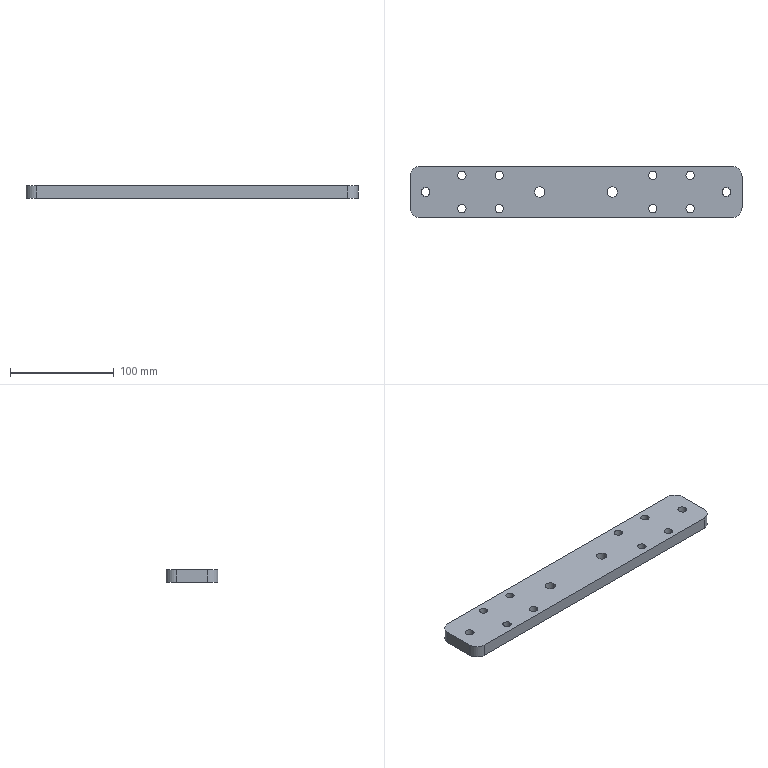Part | SolidWorks | features Extrusion 1, Fillet 1, HoleWzd 1 | 1 solid | 34 faces | box 320 x 50 x 12 mm | volume 182898 mm3 | cylinder 28 | plane 6 | commonest cylinder face diameters 8 x16 8.5 x4 10 x4 20 x4
STEP:
#1=CARTESIAN_POINT('',(10.75,25.,0.));
#2=VERTEX_POINT('',#1);
#3=CARTESIAN_POINT('',(19.25,25.,0.));
#4=VERTEX_POINT('',#3);
#5=CARTESIAN_POINT('',(15.,25.,0.));
#6=DIRECTION('',(0.,0.,1.));
#7=DIRECTION('',(1.,0.,0.));
#8=AXIS2_PLACEMENT_3D('',#5,#6,#7);
#9=CIRCLE('',#8,4.25);
#10=EDGE_CURVE('',#2,#4,#9,.T.);
#11=ORIENTED_EDGE('',*,*,#10,.F.);
#12=CARTESIAN_POINT('',(10.75,25.,12.));
#13=VERTEX_POINT('',#12);
#14=CARTESIAN_POINT('',(10.75,25.,12.));
#15=DIRECTION('',(0.,0.,1.));
#16=VECTOR('',#15,1000.);
#17=LINE('',#14,#16);
#18=EDGE_CURVE('',#2,#13,#17,.T.);
#19=ORIENTED_EDGE('',*,*,#18,.T.);
#20=CARTESIAN_POINT('',(19.25,25.,12.));
#21=VERTEX_POINT('',#20);
#22=CARTESIAN_POINT('',(15.,25.,12.));
#23=DIRECTION('',(0.,0.,1.));
#24=DIRECTION('',(1.,0.,0.));
#25=AXIS2_PLACEMENT_3D('',#22,#23,#24);
#26=CIRCLE('',#25,4.25);
#27=EDGE_CURVE('',#13,#21,#26,.T.);
#28=ORIENTED_EDGE('',*,*,#27,.T.);
#29=CARTESIAN_POINT('',(19.25,25.,12.));
#30=DIRECTION('',(0.,0.,1.));
#31=VECTOR('',#30,1000.);
#32=LINE('',#29,#31);
#33=EDGE_CURVE('',#4,#21,#32,.T.);
#34=ORIENTED_EDGE('',*,*,#33,.F.);
#35=EDGE_LOOP('',(#11,#19,#28,#34));
#36=FACE_OUTER_BOUND('',#35,.T.);
#37=CARTESIAN_POINT('',(15.,25.,12.));
#38=DIRECTION('',(0.,0.,1.));
#39=DIRECTION('',(1.,0.,0.));
#40=AXIS2_PLACEMENT_3D('',#37,#38,#39);
#41=CYLINDRICAL_SURFACE('',#40,4.25);
#42=ADVANCED_FACE('',(#36),#41,.F.);
#43=CARTESIAN_POINT('',(300.75,25.,0.));
#44=VERTEX_POINT('',#43);
#45=CARTESIAN_POINT('',(309.25,25.,0.));
#46=VERTEX_POINT('',#45);
#47=CARTESIAN_POINT('',(305.,25.,0.));
#48=DIRECTION('',(0.,0.,1.));
#49=DIRECTION('',(1.,0.,0.));
#50=AXIS2_PLACEMENT_3D('',#47,#48,#49);
#51=CIRCLE('',#50,4.25);
#52=EDGE_CURVE('',#44,#46,#51,.T.);
#53=ORIENTED_EDGE('',*,*,#52,.F.);
#54=CARTESIAN_POINT('',(300.75,25.,12.));
#55=VERTEX_POINT('',#54);
#56=CARTESIAN_POINT('',(300.75,25.,12.));
#57=DIRECTION('',(0.,0.,1.));
#58=VECTOR('',#57,1000.);
#59=LINE('',#56,#58);
#60=EDGE_CURVE('',#44,#55,#59,.T.);
#61=ORIENTED_EDGE('',*,*,#60,.T.);
#62=CARTESIAN_POINT('',(309.25,25.,12.));
#63=VERTEX_POINT('',#62);
#64=CARTESIAN_POINT('',(305.,25.,12.));
#65=DIRECTION('',(0.,0.,1.));
#66=DIRECTION('',(1.,0.,0.));
#67=AXIS2_PLACEMENT_3D('',#64,#65,#66);
#68=CIRCLE('',#67,4.25);
#69=EDGE_CURVE('',#55,#63,#68,.T.);
#70=ORIENTED_EDGE('',*,*,#69,.T.);
#71=CARTESIAN_POINT('',(309.25,25.,12.));
#72=DIRECTION('',(0.,0.,1.));
#73=VECTOR('',#72,1000.);
#74=LINE('',#71,#73);
#75=EDGE_CURVE('',#46,#63,#74,.T.);
#76=ORIENTED_EDGE('',*,*,#75,.F.);
#77=EDGE_LOOP('',(#53,#61,#70,#76));
#78=FACE_OUTER_BOUND('',#77,.T.);
#79=CARTESIAN_POINT('',(305.,25.,12.));
#80=DIRECTION('',(0.,0.,1.));
#81=DIRECTION('',(1.,0.,0.));
#82=AXIS2_PLACEMENT_3D('',#79,#80,#81);
#83=CYLINDRICAL_SURFACE('',#82,4.25);
#84=ADVANCED_FACE('',(#78),#83,.F.);
#85=CARTESIAN_POINT('',(266.,41.,12.));
#86=VERTEX_POINT('',#85);
#87=CARTESIAN_POINT('',(274.,41.,12.));
#88=VERTEX_POINT('',#87);
#89=CARTESIAN_POINT('',(270.,41.,12.));
#90=DIRECTION('',(0.,0.,1.));
#91=DIRECTION('',(-1.,0.,0.));
#92=AXIS2_PLACEMENT_3D('',#89,#90,#91);
#93=CIRCLE('',#92,4.);
#94=EDGE_CURVE('',#86,#88,#93,.T.);
#95=ORIENTED_EDGE('',*,*,#94,.T.);
#96=CARTESIAN_POINT('',(274.,41.,0.));
#97=VERTEX_POINT('',#96);
#98=CARTESIAN_POINT('',(274.,41.,12.));
#99=DIRECTION('',(0.,0.,-1.));
#100=VECTOR('',#99,1000.);
#101=LINE('',#98,#100);
#102=EDGE_CURVE('',#88,#97,#101,.T.);
#103=ORIENTED_EDGE('',*,*,#102,.T.);
#104=CARTESIAN_POINT('',(266.,41.,0.));
#105=VERTEX_POINT('',#104);
#106=CARTESIAN_POINT('',(270.,41.,0.));
#107=DIRECTION('',(0.,0.,1.));
#108=DIRECTION('',(-1.,0.,0.));
#109=AXIS2_PLACEMENT_3D('',#106,#107,#108);
#110=CIRCLE('',#109,4.);
#111=EDGE_CURVE('',#105,#97,#110,.T.);
#112=ORIENTED_EDGE('',*,*,#111,.F.);
#113=CARTESIAN_POINT('',(266.,41.,12.));
#114=DIRECTION('',(0.,0.,-1.));
#115=VECTOR('',#114,1000.);
#116=LINE('',#113,#115);
#117=EDGE_CURVE('',#86,#105,#116,.T.);
#118=ORIENTED_EDGE('',*,*,#117,.F.);
#119=EDGE_LOOP('',(#95,#103,#112,#118));
#120=FACE_OUTER_BOUND('',#119,.T.);
#121=CARTESIAN_POINT('',(270.,41.,12.));
#122=DIRECTION('',(0.,0.,-1.));
#123=DIRECTION('',(-1.,0.,0.));
#124=AXIS2_PLACEMENT_3D('',#121,#122,#123);
#125=CYLINDRICAL_SURFACE('',#124,4.);
#126=ADVANCED_FACE('',(#120),#125,.F.);
#127=CARTESIAN_POINT('',(46.,9.,12.));
#128=VERTEX_POINT('',#127);
#129=CARTESIAN_POINT('',(54.,9.,12.));
#130=VERTEX_POINT('',#129);
#131=CARTESIAN_POINT('',(50.,9.,12.));
#132=DIRECTION('',(0.,0.,1.));
#133=DIRECTION('',(-1.,0.,0.));
#134=AXIS2_PLACEMENT_3D('',#131,#132,#133);
#135=CIRCLE('',#134,4.);
#136=EDGE_CURVE('',#128,#130,#135,.T.);
#137=ORIENTED_EDGE('',*,*,#136,.T.);
#138=CARTESIAN_POINT('',(54.,9.,0.));
#139=VERTEX_POINT('',#138);
#140=CARTESIAN_POINT('',(54.,9.,12.));
#141=DIRECTION('',(0.,0.,-1.));
#142=VECTOR('',#141,1000.);
#143=LINE('',#140,#142);
#144=EDGE_CURVE('',#130,#139,#143,.T.);
#145=ORIENTED_EDGE('',*,*,#144,.T.);
#146=CARTESIAN_POINT('',(46.,9.,0.));
#147=VERTEX_POINT('',#146);
#148=CARTESIAN_POINT('',(50.,9.,0.));
#149=DIRECTION('',(0.,0.,1.));
#150=DIRECTION('',(-1.,0.,0.));
#151=AXIS2_PLACEMENT_3D('',#148,#149,#150);
#152=CIRCLE('',#151,4.);
#153=EDGE_CURVE('',#147,#139,#152,.T.);
#154=ORIENTED_EDGE('',*,*,#153,.F.);
#155=CARTESIAN_POINT('',(46.,9.,12.));
#156=DIRECTION('',(0.,0.,-1.));
#157=VECTOR('',#156,1000.);
#158=LINE('',#155,#157);
#159=EDGE_CURVE('',#128,#147,#158,.T.);
#160=ORIENTED_EDGE('',*,*,#159,.F.);
#161=EDGE_LOOP('',(#137,#145,#154,#160));
#162=FACE_OUTER_BOUND('',#161,.T.);
#163=CARTESIAN_POINT('',(50.,9.,12.));
#164=DIRECTION('',(0.,0.,-1.));
#165=DIRECTION('',(-1.,0.,0.));
#166=AXIS2_PLACEMENT_3D('',#163,#164,#165);
#167=CYLINDRICAL_SURFACE('',#166,4.);
#168=ADVANCED_FACE('',(#162),#167,.F.);
#169=CARTESIAN_POINT('',(82.,9.,12.));
#170=VERTEX_POINT('',#169);
#171=CARTESIAN_POINT('',(90.,9.,12.));
#172=VERTEX_POINT('',#171);
#173=CARTESIAN_POINT('',(86.,9.,12.));
#174=DIRECTION('',(0.,0.,1.));
#175=DIRECTION('',(-1.,0.,0.));
#176=AXIS2_PLACEMENT_3D('',#173,#174,#175);
#177=CIRCLE('',#176,4.);
#178=EDGE_CURVE('',#170,#172,#177,.T.);
#179=ORIENTED_EDGE('',*,*,#178,.T.);
#180=CARTESIAN_POINT('',(90.,9.,0.));
#181=VERTEX_POINT('',#180);
#182=CARTESIAN_POINT('',(90.,9.,12.));
#183=DIRECTION('',(0.,0.,-1.));
#184=VECTOR('',#183,1000.);
#185=LINE('',#182,#184);
#186=EDGE_CURVE('',#172,#181,#185,.T.);
#187=ORIENTED_EDGE('',*,*,#186,.T.);
#188=CARTESIAN_POINT('',(82.,9.,0.));
#189=VERTEX_POINT('',#188);
#190=CARTESIAN_POINT('',(86.,9.,0.));
#191=DIRECTION('',(0.,0.,1.));
#192=DIRECTION('',(-1.,0.,0.));
#193=AXIS2_PLACEMENT_3D('',#190,#191,#192);
#194=CIRCLE('',#193,4.);
#195=EDGE_CURVE('',#189,#181,#194,.T.);
#196=ORIENTED_EDGE('',*,*,#195,.F.);
#197=CARTESIAN_POINT('',(82.,9.,12.));
#198=DIRECTION('',(0.,0.,-1.));
#199=VECTOR('',#198,1000.);
#200=LINE('',#197,#199);
#201=EDGE_CURVE('',#170,#189,#200,.T.);
#202=ORIENTED_EDGE('',*,*,#201,.F.);
#203=EDGE_LOOP('',(#179,#187,#196,#202));
#204=FACE_OUTER_BOUND('',#203,.T.);
#205=CARTESIAN_POINT('',(86.,9.,12.));
#206=DIRECTION('',(0.,0.,-1.));
#207=DIRECTION('',(-1.,0.,0.));
#208=AXIS2_PLACEMENT_3D('',#205,#206,#207);
#209=CYLINDRICAL_SURFACE('',#208,4.);
#210=ADVANCED_FACE('',(#204),#209,.F.);
#211=CARTESIAN_POINT('',(230.,41.,12.));
#212=VERTEX_POINT('',#211);
#213=CARTESIAN_POINT('',(238.,41.,12.));
#214=VERTEX_POINT('',#213);
#215=CARTESIAN_POINT('',(234.,41.,12.));
#216=DIRECTION('',(0.,0.,1.));
#217=DIRECTION('',(-1.,0.,0.));
#218=AXIS2_PLACEMENT_3D('',#215,#216,#217);
#219=CIRCLE('',#218,4.);
#220=EDGE_CURVE('',#212,#214,#219,.T.);
#221=ORIENTED_EDGE('',*,*,#220,.T.);
#222=CARTESIAN_POINT('',(238.,41.,0.));
#223=VERTEX_POINT('',#222);
#224=CARTESIAN_POINT('',(238.,41.,12.));
#225=DIRECTION('',(0.,0.,-1.));
#226=VECTOR('',#225,1000.);
#227=LINE('',#224,#226);
#228=EDGE_CURVE('',#214,#223,#227,.T.);
#229=ORIENTED_EDGE('',*,*,#228,.T.);
#230=CARTESIAN_POINT('',(230.,41.,0.));
#231=VERTEX_POINT('',#230);
#232=CARTESIAN_POINT('',(234.,41.,0.));
#233=DIRECTION('',(0.,0.,1.));
#234=DIRECTION('',(-1.,0.,0.));
#235=AXIS2_PLACEMENT_3D('',#232,#233,#234);
#236=CIRCLE('',#235,4.);
#237=EDGE_CURVE('',#231,#223,#236,.T.);
#238=ORIENTED_EDGE('',*,*,#237,.F.);
#239=CARTESIAN_POINT('',(230.,41.,12.));
#240=DIRECTION('',(0.,0.,-1.));
#241=VECTOR('',#240,1000.);
#242=LINE('',#239,#241);
#243=EDGE_CURVE('',#212,#231,#242,.T.);
#244=ORIENTED_EDGE('',*,*,#243,.F.);
#245=EDGE_LOOP('',(#221,#229,#238,#244));
#246=FACE_OUTER_BOUND('',#245,.T.);
#247=CARTESIAN_POINT('',(234.,41.,12.));
#248=DIRECTION('',(0.,0.,-1.));
#249=DIRECTION('',(-1.,0.,0.));
#250=AXIS2_PLACEMENT_3D('',#247,#248,#249);
#251=CYLINDRICAL_SURFACE('',#250,4.);
#252=ADVANCED_FACE('',(#246),#251,.F.);
#253=CARTESIAN_POINT('',(82.,41.,12.));
#254=VERTEX_POINT('',#253);
#255=CARTESIAN_POINT('',(90.,41.,12.));
#256=VERTEX_POINT('',#255);
#257=CARTESIAN_POINT('',(86.,41.,12.));
#258=DIRECTION('',(0.,0.,1.));
#259=DIRECTION('',(1.,0.,0.));
#260=AXIS2_PLACEMENT_3D('',#257,#258,#259);
#261=CIRCLE('',#260,4.);
#262=EDGE_CURVE('',#254,#256,#261,.T.);
#263=ORIENTED_EDGE('',*,*,#262,.T.);
#264=CARTESIAN_POINT('',(90.,41.,0.));
#265=VERTEX_POINT('',#264);
#266=CARTESIAN_POINT('',(90.,41.,12.));
#267=DIRECTION('',(0.,0.,-1.));
#268=VECTOR('',#267,1000.);
#269=LINE('',#266,#268);
#270=EDGE_CURVE('',#256,#265,#269,.T.);
#271=ORIENTED_EDGE('',*,*,#270,.T.);
#272=CARTESIAN_POINT('',(82.,41.,0.));
#273=VERTEX_POINT('',#272);
#274=CARTESIAN_POINT('',(86.,41.,0.));
#275=DIRECTION('',(0.,0.,1.));
#276=DIRECTION('',(1.,0.,0.));
#277=AXIS2_PLACEMENT_3D('',#274,#275,#276);
#278=CIRCLE('',#277,4.);
#279=EDGE_CURVE('',#273,#265,#278,.T.);
#280=ORIENTED_EDGE('',*,*,#279,.F.);
#281=CARTESIAN_POINT('',(82.,41.,12.));
#282=DIRECTION('',(0.,0.,-1.));
#283=VECTOR('',#282,1000.);
#284=LINE('',#281,#283);
#285=EDGE_CURVE('',#254,#273,#284,.T.);
#286=ORIENTED_EDGE('',*,*,#285,.F.);
#287=EDGE_LOOP('',(#263,#271,#280,#286));
#288=FACE_OUTER_BOUND('',#287,.T.);
#289=CARTESIAN_POINT('',(86.,41.,12.));
#290=DIRECTION('',(0.,0.,-1.));
#291=DIRECTION('',(-1.,0.,0.));
#292=AXIS2_PLACEMENT_3D('',#289,#290,#291);
#293=CYLINDRICAL_SURFACE('',#292,4.);
#294=ADVANCED_FACE('',(#288),#293,.F.);
#295=CARTESIAN_POINT('',(46.,41.,12.));
#296=VERTEX_POINT('',#295);
#297=CARTESIAN_POINT('',(54.,41.,12.));
#298=VERTEX_POINT('',#297);
#299=CARTESIAN_POINT('',(50.,41.,12.));
#300=DIRECTION('',(0.,0.,1.));
#301=DIRECTION('',(1.,0.,0.));
#302=AXIS2_PLACEMENT_3D('',#299,#300,#301);
#303=CIRCLE('',#302,4.);
#304=EDGE_CURVE('',#296,#298,#303,.T.);
#305=ORIENTED_EDGE('',*,*,#304,.T.);
#306=CARTESIAN_POINT('',(54.,41.,0.));
#307=VERTEX_POINT('',#306);
#308=CARTESIAN_POINT('',(54.,41.,12.));
#309=DIRECTION('',(0.,0.,-1.));
#310=VECTOR('',#309,1000.);
#311=LINE('',#308,#310);
#312=EDGE_CURVE('',#298,#307,#311,.T.);
#313=ORIENTED_EDGE('',*,*,#312,.T.);
#314=CARTESIAN_POINT('',(46.,41.,0.));
#315=VERTEX_POINT('',#314);
#316=CARTESIAN_POINT('',(50.,41.,0.));
#317=DIRECTION('',(0.,0.,1.));
#318=DIRECTION('',(1.,0.,0.));
#319=AXIS2_PLACEMENT_3D('',#316,#317,#318);
#320=CIRCLE('',#319,4.);
#321=EDGE_CURVE('',#315,#307,#320,.T.);
#322=ORIENTED_EDGE('',*,*,#321,.F.);
#323=CARTESIAN_POINT('',(46.,41.,12.));
#324=DIRECTION('',(0.,0.,-1.));
#325=VECTOR('',#324,1000.);
#326=LINE('',#323,#325);
#327=EDGE_CURVE('',#296,#315,#326,.T.);
#328=ORIENTED_EDGE('',*,*,#327,.F.);
#329=EDGE_LOOP('',(#305,#313,#322,#328));
#330=FACE_OUTER_BOUND('',#329,.T.);
#331=CARTESIAN_POINT('',(50.,41.,12.));
#332=DIRECTION('',(0.,0.,-1.));
#333=DIRECTION('',(-1.,0.,0.));
#334=AXIS2_PLACEMENT_3D('',#331,#332,#333);
#335=CYLINDRICAL_SURFACE('',#334,4.);
#336=ADVANCED_FACE('',(#330),#335,.F.);
#337=CARTESIAN_POINT('',(230.,9.,12.));
#338=VERTEX_POINT('',#337);
#339=CARTESIAN_POINT('',(238.,9.,12.));
#340=VERTEX_POINT('',#339);
#341=CARTESIAN_POINT('',(234.,9.,12.));
#342=DIRECTION('',(0.,0.,1.));
#343=DIRECTION('',(1.,0.,0.));
#344=AXIS2_PLACEMENT_3D('',#341,#342,#343);
#345=CIRCLE('',#344,4.);
#346=EDGE_CURVE('',#338,#340,#345,.T.);
#347=ORIENTED_EDGE('',*,*,#346,.T.);
#348=CARTESIAN_POINT('',(238.,9.,0.));
#349=VERTEX_POINT('',#348);
#350=CARTESIAN_POINT('',(238.,9.,12.));
#351=DIRECTION('',(0.,0.,-1.));
#352=VECTOR('',#351,1000.);
#353=LINE('',#350,#352);
#354=EDGE_CURVE('',#340,#349,#353,.T.);
#355=ORIENTED_EDGE('',*,*,#354,.T.);
#356=CARTESIAN_POINT('',(230.,9.,0.));
#357=VERTEX_POINT('',#356);
#358=CARTESIAN_POINT('',(234.,9.,0.));
#359=DIRECTION('',(0.,0.,1.));
#360=DIRECTION('',(1.,0.,0.));
#361=AXIS2_PLACEMENT_3D('',#358,#359,#360);
#362=CIRCLE('',#361,4.);
#363=EDGE_CURVE('',#357,#349,#362,.T.);
#364=ORIENTED_EDGE('',*,*,#363,.F.);
#365=CARTESIAN_POINT('',(230.,9.,12.));
#366=DIRECTION('',(0.,0.,-1.));
#367=VECTOR('',#366,1000.);
#368=LINE('',#365,#367);
#369=EDGE_CURVE('',#338,#357,#368,.T.);
#370=ORIENTED_EDGE('',*,*,#369,.F.);
#371=EDGE_LOOP('',(#347,#355,#364,#370));
#372=FACE_OUTER_BOUND('',#371,.T.);
#373=CARTESIAN_POINT('',(234.,9.,12.));
#374=DIRECTION('',(0.,0.,-1.));
#375=DIRECTION('',(-1.,0.,0.));
#376=AXIS2_PLACEMENT_3D('',#373,#374,#375);
#377=CYLINDRICAL_SURFACE('',#376,4.);
#378=ADVANCED_FACE('',(#372),#377,.F.);
#379=CARTESIAN_POINT('',(190.,25.,12.));
#380=VERTEX_POINT('',#379);
#381=CARTESIAN_POINT('',(200.,25.,12.));
#382=VERTEX_POINT('',#381);
#383=CARTESIAN_POINT('',(195.,25.,12.));
#384=DIRECTION('',(0.,0.,1.));
#385=DIRECTION('',(1.,0.,0.));
#386=AXIS2_PLACEMENT_3D('',#383,#384,#385);
#387=CIRCLE('',#386,5.);
#388=EDGE_CURVE('',#380,#382,#387,.T.);
#389=ORIENTED_EDGE('',*,*,#388,.T.);
#390=CARTESIAN_POINT('',(200.,25.,0.));
#391=VERTEX_POINT('',#390);
#392=CARTESIAN_POINT('',(200.,25.,12.));
#393=DIRECTION('',(0.,0.,-1.));
#394=VECTOR('',#393,1000.);
#395=LINE('',#392,#394);
#396=EDGE_CURVE('',#382,#391,#395,.T.);
#397=ORIENTED_EDGE('',*,*,#396,.T.);
#398=CARTESIAN_POINT('',(190.,25.,0.));
#399=VERTEX_POINT('',#398);
#400=CARTESIAN_POINT('',(195.,25.,0.));
#401=DIRECTION('',(0.,0.,1.));
#402=DIRECTION('',(1.,0.,0.));
#403=AXIS2_PLACEMENT_3D('',#400,#401,#402);
#404=CIRCLE('',#403,5.);
#405=EDGE_CURVE('',#399,#391,#404,.T.);
#406=ORIENTED_EDGE('',*,*,#405,.F.);
#407=CARTESIAN_POINT('',(190.,25.,12.));
#408=DIRECTION('',(0.,0.,-1.));
#409=VECTOR('',#408,1000.);
#410=LINE('',#407,#409);
#411=EDGE_CURVE('',#380,#399,#410,.T.);
#412=ORIENTED_EDGE('',*,*,#411,.F.);
#413=EDGE_LOOP('',(#389,#397,#406,#412));
#414=FACE_OUTER_BOUND('',#413,.T.);
#415=CARTESIAN_POINT('',(195.,25.,12.));
#416=DIRECTION('',(0.,0.,-1.));
#417=DIRECTION('',(-1.,0.,0.));
#418=AXIS2_PLACEMENT_3D('',#415,#416,#417);
#419=CYLINDRICAL_SURFACE('',#418,5.);
#420=ADVANCED_FACE('',(#414),#419,.F.);
#421=CARTESIAN_POINT('',(120.,25.,12.));
#422=VERTEX_POINT('',#421);
#423=CARTESIAN_POINT('',(130.,25.,12.));
#424=VERTEX_POINT('',#423);
#425=CARTESIAN_POINT('',(125.,25.,12.));
#426=DIRECTION('',(0.,0.,1.));
#427=DIRECTION('',(1.,0.,0.));
#428=AXIS2_PLACEMENT_3D('',#425,#426,#427);
#429=CIRCLE('',#428,5.);
#430=EDGE_CURVE('',#422,#424,#429,.T.);
#431=ORIENTED_EDGE('',*,*,#430,.T.);
#432=CARTESIAN_POINT('',(130.,25.,0.));
#433=VERTEX_POINT('',#432);
#434=CARTESIAN_POINT('',(130.,25.,12.));
#435=DIRECTION('',(0.,0.,-1.));
#436=VECTOR('',#435,1000.);
#437=LINE('',#434,#436);
#438=EDGE_CURVE('',#424,#433,#437,.T.);
#439=ORIENTED_EDGE('',*,*,#438,.T.);
#440=CARTESIAN_POINT('',(120.,25.,0.));
#441=VERTEX_POINT('',#440);
#442=CARTESIAN_POINT('',(125.,25.,0.));
#443=DIRECTION('',(0.,0.,1.));
#444=DIRECTION('',(1.,0.,0.));
#445=AXIS2_PLACEMENT_3D('',#442,#443,#444);
#446=CIRCLE('',#445,5.);
#447=EDGE_CURVE('',#441,#433,#446,.T.);
#448=ORIENTED_EDGE('',*,*,#447,.F.);
#449=CARTESIAN_POINT('',(120.,25.,12.));
#450=DIRECTION('',(0.,0.,-1.));
#451=VECTOR('',#450,1000.);
#452=LINE('',#449,#451);
#453=EDGE_CURVE('',#422,#441,#452,.T.);
#454=ORIENTED_EDGE('',*,*,#453,.F.);
#455=EDGE_LOOP('',(#431,#439,#448,#454));
#456=FACE_OUTER_BOUND('',#455,.T.);
#457=CARTESIAN_POINT('',(125.,25.,12.));
#458=DIRECTION('',(0.,0.,-1.));
#459=DIRECTION('',(-1.,0.,0.));
#460=AXIS2_PLACEMENT_3D('',#457,#458,#459);
#461=CYLINDRICAL_SURFACE('',#460,5.);
#462=ADVANCED_FACE('',(#456),#461,.F.);
#463=CARTESIAN_POINT('',(266.,9.,12.));
#464=VERTEX_POINT('',#463);
#465=CARTESIAN_POINT('',(274.,9.,12.));
#466=VERTEX_POINT('',#465);
#467=CARTESIAN_POINT('',(270.,9.,12.));
#468=DIRECTION('',(0.,0.,1.));
#469=DIRECTION('',(1.,0.,0.));
#470=AXIS2_PLACEMENT_3D('',#467,#468,#469);
#471=CIRCLE('',#470,4.);
#472=EDGE_CURVE('',#464,#466,#471,.T.);
#473=ORIENTED_EDGE('',*,*,#472,.T.);
#474=CARTESIAN_POINT('',(274.,9.,0.));
#475=VERTEX_POINT('',#474);
#476=CARTESIAN_POINT('',(274.,9.,12.));
#477=DIRECTION('',(0.,0.,-1.));
#478=VECTOR('',#477,1000.);
#479=LINE('',#476,#478);
#480=EDGE_CURVE('',#466,#475,#479,.T.);
#481=ORIENTED_EDGE('',*,*,#480,.T.);
#482=CARTESIAN_POINT('',(266.,9.,0.));
#483=VERTEX_POINT('',#482);
#484=CARTESIAN_POINT('',(270.,9.,0.));
#485=DIRECTION('',(0.,0.,1.));
#486=DIRECTION('',(1.,0.,0.));
#487=AXIS2_PLACEMENT_3D('',#484,#485,#486);
#488=CIRCLE('',#487,4.);
#489=EDGE_CURVE('',#483,#475,#488,.T.);
#490=ORIENTED_EDGE('',*,*,#489,.F.);
#491=CARTESIAN_POINT('',(266.,9.,12.));
#492=DIRECTION('',(0.,0.,-1.));
#493=VECTOR('',#492,1000.);
#494=LINE('',#491,#493);
#495=EDGE_CURVE('',#464,#483,#494,.T.);
#496=ORIENTED_EDGE('',*,*,#495,.F.);
#497=EDGE_LOOP('',(#473,#481,#490,#496));
#498=FACE_OUTER_BOUND('',#497,.T.);
#499=CARTESIAN_POINT('',(270.,9.,12.));
#500=DIRECTION('',(0.,0.,-1.));
#501=DIRECTION('',(-1.,0.,0.));
#502=AXIS2_PLACEMENT_3D('',#499,#500,#501);
#503=CYLINDRICAL_SURFACE('',#502,4.);
#504=ADVANCED_FACE('',(#498),#503,.F.);
#505=CARTESIAN_POINT('',(15.,25.,12.));
#506=DIRECTION('',(0.,0.,1.));
#507=DIRECTION('',(1.,0.,0.));
#508=AXIS2_PLACEMENT_3D('',#505,#506,#507);
#509=CIRCLE('',#508,4.25);
#510=EDGE_CURVE('',#21,#13,#509,.T.);
#511=ORIENTED_EDGE('',*,*,#510,.F.);
#512=ORIENTED_EDGE('',*,*,#27,.F.);
#513=EDGE_LOOP('',(#511,#512));
#514=FACE_BOUND('',#513,.T.);
#515=CARTESIAN_POINT('',(305.,25.,12.));
#516=DIRECTION('',(0.,0.,1.));
#517=DIRECTION('',(1.,0.,0.));
#518=AXIS2_PLACEMENT_3D('',#515,#516,#517);
#519=CIRCLE('',#518,4.25);
#520=EDGE_CURVE('',#63,#55,#519,.T.);
#521=ORIENTED_EDGE('',*,*,#520,.F.);
#522=ORIENTED_EDGE('',*,*,#69,.F.);
#523=EDGE_LOOP('',(#521,#522));
#524=FACE_BOUND('',#523,.T.);
#525=ORIENTED_EDGE('',*,*,#136,.F.);
#526=CARTESIAN_POINT('',(50.,9.,12.));
#527=DIRECTION('',(0.,0.,1.));
#528=DIRECTION('',(-1.,0.,0.));
#529=AXIS2_PLACEMENT_3D('',#526,#527,#528);
#530=CIRCLE('',#529,4.);
#531=EDGE_CURVE('',#130,#128,#530,.T.);
#532=ORIENTED_EDGE('',*,*,#531,.F.);
#533=EDGE_LOOP('',(#525,#532));
#534=FACE_BOUND('',#533,.T.);
#535=ORIENTED_EDGE('',*,*,#220,.F.);
#536=CARTESIAN_POINT('',(234.,41.,12.));
#537=DIRECTION('',(0.,0.,1.));
#538=DIRECTION('',(-1.,0.,0.));
#539=AXIS2_PLACEMENT_3D('',#536,#537,#538);
#540=CIRCLE('',#539,4.);
#541=EDGE_CURVE('',#214,#212,#540,.T.);
#542=ORIENTED_EDGE('',*,*,#541,.F.);
#543=EDGE_LOOP('',(#535,#542));
#544=FACE_BOUND('',#543,.T.);
#545=ORIENTED_EDGE('',*,*,#304,.F.);
#546=CARTESIAN_POINT('',(50.,41.,12.));
#547=DIRECTION('',(0.,0.,1.));
#548=DIRECTION('',(1.,0.,0.));
#549=AXIS2_PLACEMENT_3D('',#546,#547,#548);
#550=CIRCLE('',#549,4.);
#551=EDGE_CURVE('',#298,#296,#550,.T.);
#552=ORIENTED_EDGE('',*,*,#551,.F.);
#553=EDGE_LOOP('',(#545,#552));
#554=FACE_BOUND('',#553,.T.);
#555=ORIENTED_EDGE('',*,*,#388,.F.);
#556=CARTESIAN_POINT('',(195.,25.,12.));
#557=DIRECTION('',(0.,0.,1.));
#558=DIRECTION('',(1.,0.,0.));
#559=AXIS2_PLACEMENT_3D('',#556,#557,#558);
#560=CIRCLE('',#559,5.);
#561=EDGE_CURVE('',#382,#380,#560,.T.);
#562=ORIENTED_EDGE('',*,*,#561,.F.);
#563=EDGE_LOOP('',(#555,#562));
#564=FACE_BOUND('',#563,.T.);
#565=ORIENTED_EDGE('',*,*,#472,.F.);
#566=CARTESIAN_POINT('',(270.,9.,12.));
#567=DIRECTION('',(0.,0.,1.));
#568=DIRECTION('',(1.,0.,0.));
#569=AXIS2_PLACEMENT_3D('',#566,#567,#568);
#570=CIRCLE('',#569,4.);
#571=EDGE_CURVE('',#466,#464,#570,.T.);
#572=ORIENTED_EDGE('',*,*,#571,.F.);
#573=EDGE_LOOP('',(#565,#572));
#574=FACE_BOUND('',#573,.T.);
#575=CARTESIAN_POINT('',(320.,10.,12.));
#576=VERTEX_POINT('',#575);
#577=CARTESIAN_POINT('',(320.,40.,12.));
#578=VERTEX_POINT('',#577);
#579=CARTESIAN_POINT('',(320.,0.,12.));
#580=DIRECTION('',(0.,1.,0.));
#581=VECTOR('',#580,1000.);
#582=LINE('',#579,#581);
#583=EDGE_CURVE('',#576,#578,#582,.T.);
#584=ORIENTED_EDGE('',*,*,#583,.T.);
#585=CARTESIAN_POINT('',(310.,50.,12.));
#586=VERTEX_POINT('',#585);
#587=CARTESIAN_POINT('',(310.,40.,12.));
#588=DIRECTION('',(0.,0.,1.));
#589=DIRECTION('',(1.,0.,0.));
#590=AXIS2_PLACEMENT_3D('',#587,#588,#589);
#591=CIRCLE('',#590,10.);
#592=EDGE_CURVE('',#578,#586,#591,.T.);
#593=ORIENTED_EDGE('',*,*,#592,.T.);
#594=CARTESIAN_POINT('',(10.,50.,12.));
#595=VERTEX_POINT('',#594);
#596=CARTESIAN_POINT('',(320.,50.,12.));
#597=DIRECTION('',(-1.,0.,0.));
#598=VECTOR('',#597,1000.);
#599=LINE('',#596,#598);
#600=EDGE_CURVE('',#586,#595,#599,.T.);
#601=ORIENTED_EDGE('',*,*,#600,.T.);
#602=CARTESIAN_POINT('',(0.,40.,12.));
#603=VERTEX_POINT('',#602);
#604=CARTESIAN_POINT('',(10.,40.,12.));
#605=DIRECTION('',(0.,0.,1.));
#606=DIRECTION('',(1.,0.,0.));
#607=AXIS2_PLACEMENT_3D('',#604,#605,#606);
#608=CIRCLE('',#607,10.);
#609=EDGE_CURVE('',#595,#603,#608,.T.);
#610=ORIENTED_EDGE('',*,*,#609,.T.);
#611=CARTESIAN_POINT('',(0.,10.,12.));
#612=VERTEX_POINT('',#611);
#613=CARTESIAN_POINT('',(0.,0.,12.));
#614=DIRECTION('',(0.,-1.,0.));
#615=VECTOR('',#614,1000.);
#616=LINE('',#613,#615);
#617=EDGE_CURVE('',#603,#612,#616,.T.);
#618=ORIENTED_EDGE('',*,*,#617,.T.);
#619=CARTESIAN_POINT('',(10.,0.,12.));
#620=VERTEX_POINT('',#619);
#621=CARTESIAN_POINT('',(10.,10.,12.));
#622=DIRECTION('',(0.,0.,1.));
#623=DIRECTION('',(1.,0.,0.));
#624=AXIS2_PLACEMENT_3D('',#621,#622,#623);
#625=CIRCLE('',#624,10.);
#626=EDGE_CURVE('',#612,#620,#625,.T.);
#627=ORIENTED_EDGE('',*,*,#626,.T.);
#628=CARTESIAN_POINT('',(310.,0.,12.));
#629=VERTEX_POINT('',#628);
#630=CARTESIAN_POINT('',(0.,0.,12.));
#631=DIRECTION('',(1.,0.,0.));
#632=VECTOR('',#631,1000.);
#633=LINE('',#630,#632);
#634=EDGE_CURVE('',#620,#629,#633,.T.);
#635=ORIENTED_EDGE('',*,*,#634,.T.);
#636=CARTESIAN_POINT('',(310.,10.,12.));
#637=DIRECTION('',(0.,0.,1.));
#638=DIRECTION('',(1.,0.,0.));
#639=AXIS2_PLACEMENT_3D('',#636,#637,#638);
#640=CIRCLE('',#639,10.);
#641=EDGE_CURVE('',#629,#576,#640,.T.);
#642=ORIENTED_EDGE('',*,*,#641,.T.);
#643=EDGE_LOOP('',(#584,#593,#601,#610,#618,#627,#635,#642));
#644=FACE_OUTER_BOUND('',#643,.T.);
#645=ORIENTED_EDGE('',*,*,#430,.F.);
#646=CARTESIAN_POINT('',(125.,25.,12.));
#647=DIRECTION('',(0.,0.,1.));
#648=DIRECTION('',(1.,0.,0.));
#649=AXIS2_PLACEMENT_3D('',#646,#647,#648);
#650=CIRCLE('',#649,5.);
#651=EDGE_CURVE('',#424,#422,#650,.T.);
#652=ORIENTED_EDGE('',*,*,#651,.F.);
#653=EDGE_LOOP('',(#645,#652));
#654=FACE_BOUND('',#653,.T.);
#655=ORIENTED_EDGE('',*,*,#346,.F.);
#656=CARTESIAN_POINT('',(234.,9.,12.));
#657=DIRECTION('',(0.,0.,1.));
#658=DIRECTION('',(1.,0.,0.));
#659=AXIS2_PLACEMENT_3D('',#656,#657,#658);
#660=CIRCLE('',#659,4.);
#661=EDGE_CURVE('',#340,#338,#660,.T.);
#662=ORIENTED_EDGE('',*,*,#661,.F.);
#663=EDGE_LOOP('',(#655,#662));
#664=FACE_BOUND('',#663,.T.);
#665=ORIENTED_EDGE('',*,*,#262,.F.);
#666=CARTESIAN_POINT('',(86.,41.,12.));
#667=DIRECTION('',(0.,0.,1.));
#668=DIRECTION('',(1.,0.,0.));
#669=AXIS2_PLACEMENT_3D('',#666,#667,#668);
#670=CIRCLE('',#669,4.);
#671=EDGE_CURVE('',#256,#254,#670,.T.);
#672=ORIENTED_EDGE('',*,*,#671,.F.);
#673=EDGE_LOOP('',(#665,#672));
#674=FACE_BOUND('',#673,.T.);
#675=ORIENTED_EDGE('',*,*,#178,.F.);
#676=CARTESIAN_POINT('',(86.,9.,12.));
#677=DIRECTION('',(0.,0.,1.));
#678=DIRECTION('',(-1.,0.,0.));
#679=AXIS2_PLACEMENT_3D('',#676,#677,#678);
#680=CIRCLE('',#679,4.);
#681=EDGE_CURVE('',#172,#170,#680,.T.);
#682=ORIENTED_EDGE('',*,*,#681,.F.);
#683=EDGE_LOOP('',(#675,#682));
#684=FACE_BOUND('',#683,.T.);
#685=ORIENTED_EDGE('',*,*,#94,.F.);
#686=CARTESIAN_POINT('',(270.,41.,12.));
#687=DIRECTION('',(0.,0.,1.));
#688=DIRECTION('',(-1.,0.,0.));
#689=AXIS2_PLACEMENT_3D('',#686,#687,#688);
#690=CIRCLE('',#689,4.);
#691=EDGE_CURVE('',#88,#86,#690,.T.);
#692=ORIENTED_EDGE('',*,*,#691,.F.);
#693=EDGE_LOOP('',(#685,#692));
#694=FACE_BOUND('',#693,.T.);
#695=CARTESIAN_POINT('',(0.,0.,12.));
#696=DIRECTION('',(0.,0.,1.));
#697=DIRECTION('',(1.,0.,0.));
#698=AXIS2_PLACEMENT_3D('',#695,#696,#697);
#699=PLANE('',#698);
#700=ADVANCED_FACE('',(#514,#524,#534,#544,#554,#564,#574,#644,#654,#664,#674,#684,#694),#699,.T.);
#701=CARTESIAN_POINT('',(15.,25.,0.));
#702=DIRECTION('',(0.,0.,1.));
#703=DIRECTION('',(1.,0.,0.));
#704=AXIS2_PLACEMENT_3D('',#701,#702,#703);
#705=CIRCLE('',#704,4.25);
#706=EDGE_CURVE('',#4,#2,#705,.T.);
#707=ORIENTED_EDGE('',*,*,#706,.T.);
#708=ORIENTED_EDGE('',*,*,#10,.T.);
#709=EDGE_LOOP('',(#707,#708));
#710=FACE_BOUND('',#709,.T.);
#711=CARTESIAN_POINT('',(305.,25.,0.));
#712=DIRECTION('',(0.,0.,1.));
#713=DIRECTION('',(1.,0.,0.));
#714=AXIS2_PLACEMENT_3D('',#711,#712,#713);
#715=CIRCLE('',#714,4.25);
#716=EDGE_CURVE('',#46,#44,#715,.T.);
#717=ORIENTED_EDGE('',*,*,#716,.T.);
#718=ORIENTED_EDGE('',*,*,#52,.T.);
#719=EDGE_LOOP('',(#717,#718));
#720=FACE_BOUND('',#719,.T.);
#721=CARTESIAN_POINT('',(310.,50.,0.));
#722=VERTEX_POINT('',#721);
#723=CARTESIAN_POINT('',(10.,50.,0.));
#724=VERTEX_POINT('',#723);
#725=CARTESIAN_POINT('',(320.,50.,0.));
#726=DIRECTION('',(-1.,0.,0.));
#727=VECTOR('',#726,1000.);
#728=LINE('',#725,#727);
#729=EDGE_CURVE('',#722,#724,#728,.T.);
#730=ORIENTED_EDGE('',*,*,#729,.F.);
#731=CARTESIAN_POINT('',(320.,40.,0.));
#732=VERTEX_POINT('',#731);
#733=CARTESIAN_POINT('',(310.,40.,0.));
#734=DIRECTION('',(0.,0.,-1.));
#735=DIRECTION('',(1.,0.,0.));
#736=AXIS2_PLACEMENT_3D('',#733,#734,#735);
#737=CIRCLE('',#736,10.);
#738=EDGE_CURVE('',#722,#732,#737,.T.);
#739=ORIENTED_EDGE('',*,*,#738,.T.);
#740=CARTESIAN_POINT('',(320.,10.,0.));
#741=VERTEX_POINT('',#740);
#742=CARTESIAN_POINT('',(320.,0.,0.));
#743=DIRECTION('',(0.,1.,0.));
#744=VECTOR('',#743,1000.);
#745=LINE('',#742,#744);
#746=EDGE_CURVE('',#741,#732,#745,.T.);
#747=ORIENTED_EDGE('',*,*,#746,.F.);
#748=CARTESIAN_POINT('',(310.,0.,0.));
#749=VERTEX_POINT('',#748);
#750=CARTESIAN_POINT('',(310.,10.,0.));
#751=DIRECTION('',(0.,0.,-1.));
#752=DIRECTION('',(1.,0.,0.));
#753=AXIS2_PLACEMENT_3D('',#750,#751,#752);
#754=CIRCLE('',#753,10.);
#755=EDGE_CURVE('',#741,#749,#754,.T.);
#756=ORIENTED_EDGE('',*,*,#755,.T.);
#757=CARTESIAN_POINT('',(10.,0.,0.));
#758=VERTEX_POINT('',#757);
#759=CARTESIAN_POINT('',(0.,0.,0.));
#760=DIRECTION('',(1.,0.,0.));
#761=VECTOR('',#760,1000.);
#762=LINE('',#759,#761);
#763=EDGE_CURVE('',#758,#749,#762,.T.);
#764=ORIENTED_EDGE('',*,*,#763,.F.);
#765=CARTESIAN_POINT('',(0.,10.,0.));
#766=VERTEX_POINT('',#765);
#767=CARTESIAN_POINT('',(10.,10.,0.));
#768=DIRECTION('',(0.,0.,-1.));
#769=DIRECTION('',(1.,0.,0.));
#770=AXIS2_PLACEMENT_3D('',#767,#768,#769);
#771=CIRCLE('',#770,10.);
#772=EDGE_CURVE('',#758,#766,#771,.T.);
#773=ORIENTED_EDGE('',*,*,#772,.T.);
#774=CARTESIAN_POINT('',(0.,40.,0.));
#775=VERTEX_POINT('',#774);
#776=CARTESIAN_POINT('',(0.,0.,0.));
#777=DIRECTION('',(0.,-1.,0.));
#778=VECTOR('',#777,1000.);
#779=LINE('',#776,#778);
#780=EDGE_CURVE('',#775,#766,#779,.T.);
#781=ORIENTED_EDGE('',*,*,#780,.F.);
#782=CARTESIAN_POINT('',(10.,40.,0.));
#783=DIRECTION('',(0.,0.,-1.));
#784=DIRECTION('',(1.,0.,0.));
#785=AXIS2_PLACEMENT_3D('',#782,#783,#784);
#786=CIRCLE('',#785,10.);
#787=EDGE_CURVE('',#775,#724,#786,.T.);
#788=ORIENTED_EDGE('',*,*,#787,.T.);
#789=EDGE_LOOP('',(#730,#739,#747,#756,#764,#773,#781,#788));
#790=FACE_OUTER_BOUND('',#789,.T.);
#791=ORIENTED_EDGE('',*,*,#489,.T.);
#792=CARTESIAN_POINT('',(270.,9.,0.));
#793=DIRECTION('',(0.,0.,1.));
#794=DIRECTION('',(1.,0.,0.));
#795=AXIS2_PLACEMENT_3D('',#792,#793,#794);
#796=CIRCLE('',#795,4.);
#797=EDGE_CURVE('',#475,#483,#796,.T.);
#798=ORIENTED_EDGE('',*,*,#797,.T.);
#799=EDGE_LOOP('',(#791,#798));
#800=FACE_BOUND('',#799,.T.);
#801=ORIENTED_EDGE('',*,*,#447,.T.);
#802=CARTESIAN_POINT('',(125.,25.,0.));
#803=DIRECTION('',(0.,0.,1.));
#804=DIRECTION('',(1.,0.,0.));
#805=AXIS2_PLACEMENT_3D('',#802,#803,#804);
#806=CIRCLE('',#805,5.);
#807=EDGE_CURVE('',#433,#441,#806,.T.);
#808=ORIENTED_EDGE('',*,*,#807,.T.);
#809=EDGE_LOOP('',(#801,#808));
#810=FACE_BOUND('',#809,.T.);
#811=ORIENTED_EDGE('',*,*,#405,.T.);
#812=CARTESIAN_POINT('',(195.,25.,0.));
#813=DIRECTION('',(0.,0.,1.));
#814=DIRECTION('',(1.,0.,0.));
#815=AXIS2_PLACEMENT_3D('',#812,#813,#814);
#816=CIRCLE('',#815,5.);
#817=EDGE_CURVE('',#391,#399,#816,.T.);
#818=ORIENTED_EDGE('',*,*,#817,.T.);
#819=EDGE_LOOP('',(#811,#818));
#820=FACE_BOUND('',#819,.T.);
#821=ORIENTED_EDGE('',*,*,#363,.T.);
#822=CARTESIAN_POINT('',(234.,9.,0.));
#823=DIRECTION('',(0.,0.,1.));
#824=DIRECTION('',(1.,0.,0.));
#825=AXIS2_PLACEMENT_3D('',#822,#823,#824);
#826=CIRCLE('',#825,4.);
#827=EDGE_CURVE('',#349,#357,#826,.T.);
#828=ORIENTED_EDGE('',*,*,#827,.T.);
#829=EDGE_LOOP('',(#821,#828));
#830=FACE_BOUND('',#829,.T.);
#831=ORIENTED_EDGE('',*,*,#321,.T.);
#832=CARTESIAN_POINT('',(50.,41.,0.));
#833=DIRECTION('',(0.,0.,1.));
#834=DIRECTION('',(1.,0.,0.));
#835=AXIS2_PLACEMENT_3D('',#832,#833,#834);
#836=CIRCLE('',#835,4.);
#837=EDGE_CURVE('',#307,#315,#836,.T.);
#838=ORIENTED_EDGE('',*,*,#837,.T.);
#839=EDGE_LOOP('',(#831,#838));
#840=FACE_BOUND('',#839,.T.);
#841=ORIENTED_EDGE('',*,*,#279,.T.);
#842=CARTESIAN_POINT('',(86.,41.,0.));
#843=DIRECTION('',(0.,0.,1.));
#844=DIRECTION('',(1.,0.,0.));
#845=AXIS2_PLACEMENT_3D('',#842,#843,#844);
#846=CIRCLE('',#845,4.);
#847=EDGE_CURVE('',#265,#273,#846,.T.);
#848=ORIENTED_EDGE('',*,*,#847,.T.);
#849=EDGE_LOOP('',(#841,#848));
#850=FACE_BOUND('',#849,.T.);
#851=ORIENTED_EDGE('',*,*,#237,.T.);
#852=CARTESIAN_POINT('',(234.,41.,0.));
#853=DIRECTION('',(0.,0.,1.));
#854=DIRECTION('',(-1.,0.,0.));
#855=AXIS2_PLACEMENT_3D('',#852,#853,#854);
#856=CIRCLE('',#855,4.);
#857=EDGE_CURVE('',#223,#231,#856,.T.);
#858=ORIENTED_EDGE('',*,*,#857,.T.);
#859=EDGE_LOOP('',(#851,#858));
#860=FACE_BOUND('',#859,.T.);
#861=ORIENTED_EDGE('',*,*,#195,.T.);
#862=CARTESIAN_POINT('',(86.,9.,0.));
#863=DIRECTION('',(0.,0.,1.));
#864=DIRECTION('',(-1.,0.,0.));
#865=AXIS2_PLACEMENT_3D('',#862,#863,#864);
#866=CIRCLE('',#865,4.);
#867=EDGE_CURVE('',#181,#189,#866,.T.);
#868=ORIENTED_EDGE('',*,*,#867,.T.);
#869=EDGE_LOOP('',(#861,#868));
#870=FACE_BOUND('',#869,.T.);
#871=ORIENTED_EDGE('',*,*,#153,.T.);
#872=CARTESIAN_POINT('',(50.,9.,0.));
#873=DIRECTION('',(0.,0.,1.));
#874=DIRECTION('',(-1.,0.,0.));
#875=AXIS2_PLACEMENT_3D('',#872,#873,#874);
#876=CIRCLE('',#875,4.);
#877=EDGE_CURVE('',#139,#147,#876,.T.);
#878=ORIENTED_EDGE('',*,*,#877,.T.);
#879=EDGE_LOOP('',(#871,#878));
#880=FACE_BOUND('',#879,.T.);
#881=ORIENTED_EDGE('',*,*,#111,.T.);
#882=CARTESIAN_POINT('',(270.,41.,0.));
#883=DIRECTION('',(0.,0.,1.));
#884=DIRECTION('',(-1.,0.,0.));
#885=AXIS2_PLACEMENT_3D('',#882,#883,#884);
#886=CIRCLE('',#885,4.);
#887=EDGE_CURVE('',#97,#105,#886,.T.);
#888=ORIENTED_EDGE('',*,*,#887,.T.);
#889=EDGE_LOOP('',(#881,#888));
#890=FACE_BOUND('',#889,.T.);
#891=CARTESIAN_POINT('',(0.,0.,0.));
#892=DIRECTION('',(0.,0.,1.));
#893=DIRECTION('',(1.,0.,0.));
#894=AXIS2_PLACEMENT_3D('',#891,#892,#893);
#895=PLANE('',#894);
#896=ADVANCED_FACE('',(#710,#720,#790,#800,#810,#820,#830,#840,#850,#860,#870,#880,#890),#895,.F.);
#897=ORIENTED_EDGE('',*,*,#746,.T.);
#898=CARTESIAN_POINT('',(320.,40.,12.));
#899=DIRECTION('',(0.,0.,1.));
#900=VECTOR('',#899,1000.);
#901=LINE('',#898,#900);
#902=EDGE_CURVE('',#732,#578,#901,.T.);
#903=ORIENTED_EDGE('',*,*,#902,.T.);
#904=ORIENTED_EDGE('',*,*,#583,.F.);
#905=CARTESIAN_POINT('',(320.,10.,12.));
#906=DIRECTION('',(0.,0.,-1.));
#907=VECTOR('',#906,1000.);
#908=LINE('',#905,#907);
#909=EDGE_CURVE('',#576,#741,#908,.T.);
#910=ORIENTED_EDGE('',*,*,#909,.T.);
#911=EDGE_LOOP('',(#897,#903,#904,#910));
#912=FACE_OUTER_BOUND('',#911,.T.);
#913=CARTESIAN_POINT('',(320.,0.,12.));
#914=DIRECTION('',(-1.,0.,0.));
#915=DIRECTION('',(0.,0.,1.));
#916=AXIS2_PLACEMENT_3D('',#913,#914,#915);
#917=PLANE('',#916);
#918=ADVANCED_FACE('',(#912),#917,.F.);
#919=ORIENTED_EDGE('',*,*,#600,.F.);
#920=CARTESIAN_POINT('',(310.,50.,12.));
#921=DIRECTION('',(0.,0.,-1.));
#922=VECTOR('',#921,1000.);
#923=LINE('',#920,#922);
#924=EDGE_CURVE('',#586,#722,#923,.T.);
#925=ORIENTED_EDGE('',*,*,#924,.T.);
#926=ORIENTED_EDGE('',*,*,#729,.T.);
#927=CARTESIAN_POINT('',(10.,50.,12.));
#928=DIRECTION('',(0.,0.,1.));
#929=VECTOR('',#928,1000.);
#930=LINE('',#927,#929);
#931=EDGE_CURVE('',#724,#595,#930,.T.);
#932=ORIENTED_EDGE('',*,*,#931,.T.);
#933=EDGE_LOOP('',(#919,#925,#926,#932));
#934=FACE_OUTER_BOUND('',#933,.T.);
#935=CARTESIAN_POINT('',(320.,50.,12.));
#936=DIRECTION('',(0.,-1.,0.));
#937=DIRECTION('',(1.,0.,0.));
#938=AXIS2_PLACEMENT_3D('',#935,#936,#937);
#939=PLANE('',#938);
#940=ADVANCED_FACE('',(#934),#939,.F.);
#941=ORIENTED_EDGE('',*,*,#617,.F.);
#942=CARTESIAN_POINT('',(0.,40.,12.));
#943=DIRECTION('',(0.,0.,-1.));
#944=VECTOR('',#943,1000.);
#945=LINE('',#942,#944);
#946=EDGE_CURVE('',#603,#775,#945,.T.);
#947=ORIENTED_EDGE('',*,*,#946,.T.);
#948=ORIENTED_EDGE('',*,*,#780,.T.);
#949=CARTESIAN_POINT('',(0.,10.,12.));
#950=DIRECTION('',(0.,0.,1.));
#951=VECTOR('',#950,1000.);
#952=LINE('',#949,#951);
#953=EDGE_CURVE('',#766,#612,#952,.T.);
#954=ORIENTED_EDGE('',*,*,#953,.T.);
#955=EDGE_LOOP('',(#941,#947,#948,#954));
#956=FACE_OUTER_BOUND('',#955,.T.);
#957=CARTESIAN_POINT('',(0.,0.,12.));
#958=DIRECTION('',(1.,0.,0.));
#959=DIRECTION('',(0.,0.,-1.));
#960=AXIS2_PLACEMENT_3D('',#957,#958,#959);
#961=PLANE('',#960);
#962=ADVANCED_FACE('',(#956),#961,.F.);
#963=ORIENTED_EDGE('',*,*,#763,.T.);
#964=CARTESIAN_POINT('',(310.,0.,12.));
#965=DIRECTION('',(0.,0.,1.));
#966=VECTOR('',#965,1000.);
#967=LINE('',#964,#966);
#968=EDGE_CURVE('',#749,#629,#967,.T.);
#969=ORIENTED_EDGE('',*,*,#968,.T.);
#970=ORIENTED_EDGE('',*,*,#634,.F.);
#971=CARTESIAN_POINT('',(10.,0.,12.));
#972=DIRECTION('',(0.,0.,-1.));
#973=VECTOR('',#972,1000.);
#974=LINE('',#971,#973);
#975=EDGE_CURVE('',#620,#758,#974,.T.);
#976=ORIENTED_EDGE('',*,*,#975,.T.);
#977=EDGE_LOOP('',(#963,#969,#970,#976));
#978=FACE_OUTER_BOUND('',#977,.T.);
#979=CARTESIAN_POINT('',(0.,0.,12.));
#980=DIRECTION('',(0.,1.,0.));
#981=DIRECTION('',(-1.,0.,0.));
#982=AXIS2_PLACEMENT_3D('',#979,#980,#981);
#983=PLANE('',#982);
#984=ADVANCED_FACE('',(#978),#983,.F.);
#985=ORIENTED_EDGE('',*,*,#480,.F.);
#986=ORIENTED_EDGE('',*,*,#571,.T.);
#987=ORIENTED_EDGE('',*,*,#495,.T.);
#988=ORIENTED_EDGE('',*,*,#797,.F.);
#989=EDGE_LOOP('',(#985,#986,#987,#988));
#990=FACE_OUTER_BOUND('',#989,.T.);
#991=CARTESIAN_POINT('',(270.,9.,12.));
#992=DIRECTION('',(0.,0.,-1.));
#993=DIRECTION('',(-1.,0.,0.));
#994=AXIS2_PLACEMENT_3D('',#991,#992,#993);
#995=CYLINDRICAL_SURFACE('',#994,4.);
#996=ADVANCED_FACE('',(#990),#995,.F.);
#997=ORIENTED_EDGE('',*,*,#438,.F.);
#998=ORIENTED_EDGE('',*,*,#651,.T.);
#999=ORIENTED_EDGE('',*,*,#453,.T.);
#1000=ORIENTED_EDGE('',*,*,#807,.F.);
#1001=EDGE_LOOP('',(#997,#998,#999,#1000));
#1002=FACE_OUTER_BOUND('',#1001,.T.);
#1003=CARTESIAN_POINT('',(125.,25.,12.));
#1004=DIRECTION('',(0.,0.,-1.));
#1005=DIRECTION('',(-1.,0.,0.));
#1006=AXIS2_PLACEMENT_3D('',#1003,#1004,#1005);
#1007=CYLINDRICAL_SURFACE('',#1006,5.);
#1008=ADVANCED_FACE('',(#1002),#1007,.F.);
#1009=ORIENTED_EDGE('',*,*,#396,.F.);
#1010=ORIENTED_EDGE('',*,*,#561,.T.);
#1011=ORIENTED_EDGE('',*,*,#411,.T.);
#1012=ORIENTED_EDGE('',*,*,#817,.F.);
#1013=EDGE_LOOP('',(#1009,#1010,#1011,#1012));
#1014=FACE_OUTER_BOUND('',#1013,.T.);
#1015=CARTESIAN_POINT('',(195.,25.,12.));
#1016=DIRECTION('',(0.,0.,-1.));
#1017=DIRECTION('',(-1.,0.,0.));
#1018=AXIS2_PLACEMENT_3D('',#1015,#1016,#1017);
#1019=CYLINDRICAL_SURFACE('',#1018,5.);
#1020=ADVANCED_FACE('',(#1014),#1019,.F.);
#1021=ORIENTED_EDGE('',*,*,#354,.F.);
#1022=ORIENTED_EDGE('',*,*,#661,.T.);
#1023=ORIENTED_EDGE('',*,*,#369,.T.);
#1024=ORIENTED_EDGE('',*,*,#827,.F.);
#1025=EDGE_LOOP('',(#1021,#1022,#1023,#1024));
#1026=FACE_OUTER_BOUND('',#1025,.T.);
#1027=CARTESIAN_POINT('',(234.,9.,12.));
#1028=DIRECTION('',(0.,0.,-1.));
#1029=DIRECTION('',(-1.,0.,0.));
#1030=AXIS2_PLACEMENT_3D('',#1027,#1028,#1029);
#1031=CYLINDRICAL_SURFACE('',#1030,4.);
#1032=ADVANCED_FACE('',(#1026),#1031,.F.);
#1033=ORIENTED_EDGE('',*,*,#312,.F.);
#1034=ORIENTED_EDGE('',*,*,#551,.T.);
#1035=ORIENTED_EDGE('',*,*,#327,.T.);
#1036=ORIENTED_EDGE('',*,*,#837,.F.);
#1037=EDGE_LOOP('',(#1033,#1034,#1035,#1036));
#1038=FACE_OUTER_BOUND('',#1037,.T.);
#1039=CARTESIAN_POINT('',(50.,41.,12.));
#1040=DIRECTION('',(0.,0.,-1.));
#1041=DIRECTION('',(-1.,0.,0.));
#1042=AXIS2_PLACEMENT_3D('',#1039,#1040,#1041);
#1043=CYLINDRICAL_SURFACE('',#1042,4.);
#1044=ADVANCED_FACE('',(#1038),#1043,.F.);
#1045=ORIENTED_EDGE('',*,*,#270,.F.);
#1046=ORIENTED_EDGE('',*,*,#671,.T.);
#1047=ORIENTED_EDGE('',*,*,#285,.T.);
#1048=ORIENTED_EDGE('',*,*,#847,.F.);
#1049=EDGE_LOOP('',(#1045,#1046,#1047,#1048));
#1050=FACE_OUTER_BOUND('',#1049,.T.);
#1051=CARTESIAN_POINT('',(86.,41.,12.));
#1052=DIRECTION('',(0.,0.,-1.));
#1053=DIRECTION('',(-1.,0.,0.));
#1054=AXIS2_PLACEMENT_3D('',#1051,#1052,#1053);
#1055=CYLINDRICAL_SURFACE('',#1054,4.);
#1056=ADVANCED_FACE('',(#1050),#1055,.F.);
#1057=ORIENTED_EDGE('',*,*,#228,.F.);
#1058=ORIENTED_EDGE('',*,*,#541,.T.);
#1059=ORIENTED_EDGE('',*,*,#243,.T.);
#1060=ORIENTED_EDGE('',*,*,#857,.F.);
#1061=EDGE_LOOP('',(#1057,#1058,#1059,#1060));
#1062=FACE_OUTER_BOUND('',#1061,.T.);
#1063=CARTESIAN_POINT('',(234.,41.,12.));
#1064=DIRECTION('',(0.,0.,-1.));
#1065=DIRECTION('',(-1.,0.,0.));
#1066=AXIS2_PLACEMENT_3D('',#1063,#1064,#1065);
#1067=CYLINDRICAL_SURFACE('',#1066,4.);
#1068=ADVANCED_FACE('',(#1062),#1067,.F.);
#1069=ORIENTED_EDGE('',*,*,#186,.F.);
#1070=ORIENTED_EDGE('',*,*,#681,.T.);
#1071=ORIENTED_EDGE('',*,*,#201,.T.);
#1072=ORIENTED_EDGE('',*,*,#867,.F.);
#1073=EDGE_LOOP('',(#1069,#1070,#1071,#1072));
#1074=FACE_OUTER_BOUND('',#1073,.T.);
#1075=CARTESIAN_POINT('',(86.,9.,12.));
#1076=DIRECTION('',(0.,0.,-1.));
#1077=DIRECTION('',(-1.,0.,0.));
#1078=AXIS2_PLACEMENT_3D('',#1075,#1076,#1077);
#1079=CYLINDRICAL_SURFACE('',#1078,4.);
#1080=ADVANCED_FACE('',(#1074),#1079,.F.);
#1081=ORIENTED_EDGE('',*,*,#144,.F.);
#1082=ORIENTED_EDGE('',*,*,#531,.T.);
#1083=ORIENTED_EDGE('',*,*,#159,.T.);
#1084=ORIENTED_EDGE('',*,*,#877,.F.);
#1085=EDGE_LOOP('',(#1081,#1082,#1083,#1084));
#1086=FACE_OUTER_BOUND('',#1085,.T.);
#1087=CARTESIAN_POINT('',(50.,9.,12.));
#1088=DIRECTION('',(0.,0.,-1.));
#1089=DIRECTION('',(-1.,0.,0.));
#1090=AXIS2_PLACEMENT_3D('',#1087,#1088,#1089);
#1091=CYLINDRICAL_SURFACE('',#1090,4.);
#1092=ADVANCED_FACE('',(#1086),#1091,.F.);
#1093=ORIENTED_EDGE('',*,*,#102,.F.);
#1094=ORIENTED_EDGE('',*,*,#691,.T.);
#1095=ORIENTED_EDGE('',*,*,#117,.T.);
#1096=ORIENTED_EDGE('',*,*,#887,.F.);
#1097=EDGE_LOOP('',(#1093,#1094,#1095,#1096));
#1098=FACE_OUTER_BOUND('',#1097,.T.);
#1099=CARTESIAN_POINT('',(270.,41.,12.));
#1100=DIRECTION('',(0.,0.,-1.));
#1101=DIRECTION('',(-1.,0.,0.));
#1102=AXIS2_PLACEMENT_3D('',#1099,#1100,#1101);
#1103=CYLINDRICAL_SURFACE('',#1102,4.);
#1104=ADVANCED_FACE('',(#1098),#1103,.F.);
#1105=ORIENTED_EDGE('',*,*,#60,.F.);
#1106=ORIENTED_EDGE('',*,*,#716,.F.);
#1107=ORIENTED_EDGE('',*,*,#75,.T.);
#1108=ORIENTED_EDGE('',*,*,#520,.T.);
#1109=EDGE_LOOP('',(#1105,#1106,#1107,#1108));
#1110=FACE_OUTER_BOUND('',#1109,.T.);
#1111=CARTESIAN_POINT('',(305.,25.,12.));
#1112=DIRECTION('',(0.,0.,1.));
#1113=DIRECTION('',(1.,0.,0.));
#1114=AXIS2_PLACEMENT_3D('',#1111,#1112,#1113);
#1115=CYLINDRICAL_SURFACE('',#1114,4.25);
#1116=ADVANCED_FACE('',(#1110),#1115,.F.);
#1117=ORIENTED_EDGE('',*,*,#18,.F.);
#1118=ORIENTED_EDGE('',*,*,#706,.F.);
#1119=ORIENTED_EDGE('',*,*,#33,.T.);
#1120=ORIENTED_EDGE('',*,*,#510,.T.);
#1121=EDGE_LOOP('',(#1117,#1118,#1119,#1120));
#1122=FACE_OUTER_BOUND('',#1121,.T.);
#1123=CARTESIAN_POINT('',(15.,25.,12.));
#1124=DIRECTION('',(0.,0.,1.));
#1125=DIRECTION('',(1.,0.,0.));
#1126=AXIS2_PLACEMENT_3D('',#1123,#1124,#1125);
#1127=CYLINDRICAL_SURFACE('',#1126,4.25);
#1128=ADVANCED_FACE('',(#1122),#1127,.F.);
#1129=ORIENTED_EDGE('',*,*,#592,.F.);
#1130=ORIENTED_EDGE('',*,*,#902,.F.);
#1131=ORIENTED_EDGE('',*,*,#738,.F.);
#1132=ORIENTED_EDGE('',*,*,#924,.F.);
#1133=EDGE_LOOP('',(#1129,#1130,#1131,#1132));
#1134=FACE_OUTER_BOUND('',#1133,.T.);
#1135=CARTESIAN_POINT('',(310.,40.,12.));
#1136=DIRECTION('',(0.,0.,-1.));
#1137=DIRECTION('',(-1.,0.,0.));
#1138=AXIS2_PLACEMENT_3D('',#1135,#1136,#1137);
#1139=CYLINDRICAL_SURFACE('',#1138,10.);
#1140=ADVANCED_FACE('',(#1134),#1139,.T.);
#1141=ORIENTED_EDGE('',*,*,#641,.F.);
#1142=ORIENTED_EDGE('',*,*,#968,.F.);
#1143=ORIENTED_EDGE('',*,*,#755,.F.);
#1144=ORIENTED_EDGE('',*,*,#909,.F.);
#1145=EDGE_LOOP('',(#1141,#1142,#1143,#1144));
#1146=FACE_OUTER_BOUND('',#1145,.T.);
#1147=CARTESIAN_POINT('',(310.,10.,12.));
#1148=DIRECTION('',(0.,0.,-1.));
#1149=DIRECTION('',(-1.,0.,0.));
#1150=AXIS2_PLACEMENT_3D('',#1147,#1148,#1149);
#1151=CYLINDRICAL_SURFACE('',#1150,10.);
#1152=ADVANCED_FACE('',(#1146),#1151,.T.);
#1153=ORIENTED_EDGE('',*,*,#609,.F.);
#1154=ORIENTED_EDGE('',*,*,#931,.F.);
#1155=ORIENTED_EDGE('',*,*,#787,.F.);
#1156=ORIENTED_EDGE('',*,*,#946,.F.);
#1157=EDGE_LOOP('',(#1153,#1154,#1155,#1156));
#1158=FACE_OUTER_BOUND('',#1157,.T.);
#1159=CARTESIAN_POINT('',(10.,40.,12.));
#1160=DIRECTION('',(0.,0.,-1.));
#1161=DIRECTION('',(-1.,0.,0.));
#1162=AXIS2_PLACEMENT_3D('',#1159,#1160,#1161);
#1163=CYLINDRICAL_SURFACE('',#1162,10.);
#1164=ADVANCED_FACE('',(#1158),#1163,.T.);
#1165=ORIENTED_EDGE('',*,*,#626,.F.);
#1166=ORIENTED_EDGE('',*,*,#953,.F.);
#1167=ORIENTED_EDGE('',*,*,#772,.F.);
#1168=ORIENTED_EDGE('',*,*,#975,.F.);
#1169=EDGE_LOOP('',(#1165,#1166,#1167,#1168));
#1170=FACE_OUTER_BOUND('',#1169,.T.);
#1171=CARTESIAN_POINT('',(10.,10.,12.));
#1172=DIRECTION('',(0.,0.,-1.));
#1173=DIRECTION('',(-1.,0.,0.));
#1174=AXIS2_PLACEMENT_3D('',#1171,#1172,#1173);
#1175=CYLINDRICAL_SURFACE('',#1174,10.);
#1176=ADVANCED_FACE('',(#1170),#1175,.T.);
#1177=CLOSED_SHELL('',(#42,#84,#126,#168,#210,#252,#294,#336,#378,#420,#462,#504,#700,#896,#918,#940,#962,#984,#996,#1008,#1020,#1032,#1044,#1056,#1068,#1080,#1092,#1104,#1116,#1128,#1140,#1152,#1164,#1176));
#1178=MANIFOLD_SOLID_BREP('',#1177);
#1179=CARTESIAN_POINT('',(0.,0.,0.));
#1180=DIRECTION('',(0.,0.,1.));
#1181=DIRECTION('',(1.,0.,0.));
#1182=AXIS2_PLACEMENT_3D('',#1179,#1180,#1181);
#1183=(LENGTH_UNIT()NAMED_UNIT(*)SI_UNIT(.MILLI.,.METRE.));
#1184=UNCERTAINTY_MEASURE_WITH_UNIT(LENGTH_MEASURE(0.00001),#1183,'','');
#1185=(NAMED_UNIT(*)PLANE_ANGLE_UNIT()SI_UNIT($,.RADIAN.));
#1186=(NAMED_UNIT(*)SI_UNIT($,.STERADIAN.)SOLID_ANGLE_UNIT());
#1187=(GEOMETRIC_REPRESENTATION_CONTEXT(3)GLOBAL_UNCERTAINTY_ASSIGNED_CONTEXT((#1184))GLOBAL_UNIT_ASSIGNED_CONTEXT((#1183,#1185,#1186))REPRESENTATION_CONTEXT('',''));
#1188=ADVANCED_BREP_SHAPE_REPRESENTATION('',(#1178,#1182),#1187);